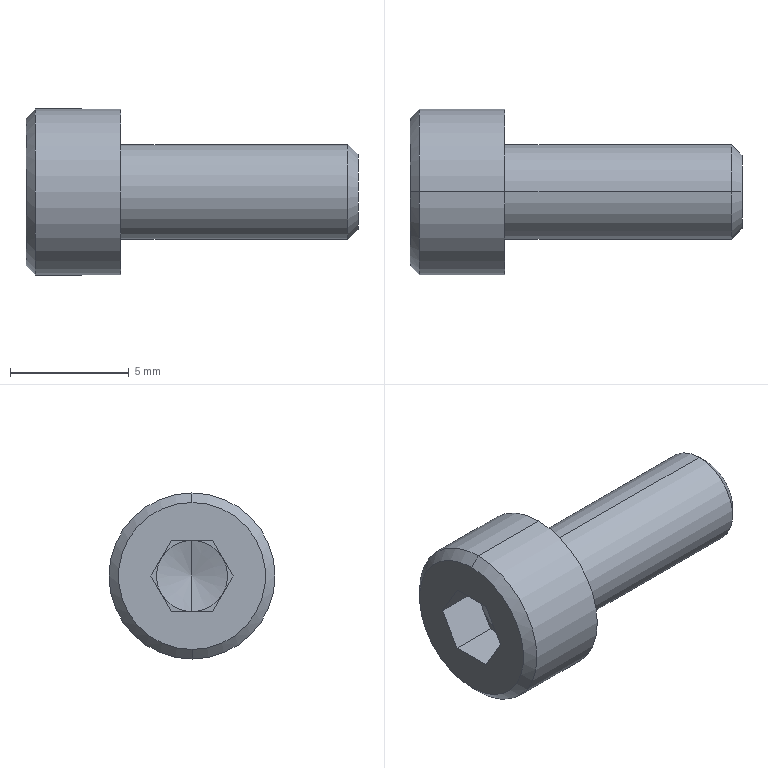Part | STEP file | 0230_302_SCB4-10 | 1 solid | 25 faces | box 14 x 7 x 7 mm | volume 260.298 mm3 | plane 15 | cone 6 | cylinder 4 | commonest cylinder face diameters 4 x2 7 x2